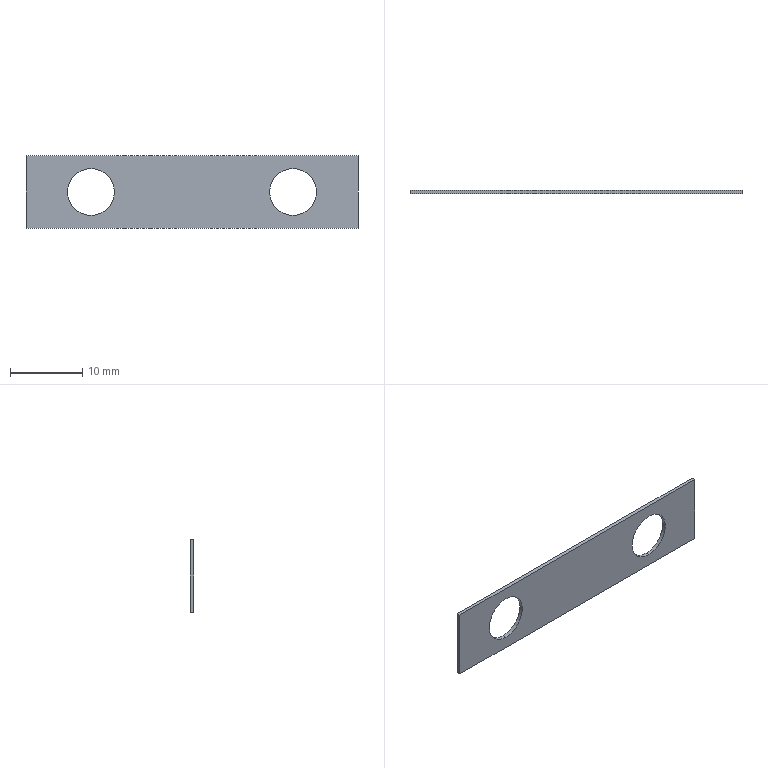Part | SolidWorks | features BaseBody 1 | 1 solid | 10 faces | box 46 x 0.5 x 10 mm | volume 196.817 mm3 | plane 6 | cylinder 4 | commonest cylinder face diameters 6.5 x4
STEP:
#1=CARTESIAN_POINT('',(14.,0.5,3.25));
#2=VERTEX_POINT('',#1);
#3=CARTESIAN_POINT('',(14.,0.5,-3.25));
#4=VERTEX_POINT('',#3);
#5=CARTESIAN_POINT('',(14.,0.5,0.));
#6=DIRECTION('',(0.,-1.,0.));
#7=DIRECTION('',(0.,0.,1.));
#8=AXIS2_PLACEMENT_3D('',#5,#6,#7);
#9=CIRCLE('',#8,3.25);
#10=EDGE_CURVE('',#2,#4,#9,.T.);
#11=ORIENTED_EDGE('',*,*,#10,.T.);
#12=CARTESIAN_POINT('',(14.,0.5,0.));
#13=DIRECTION('',(0.,-1.,0.));
#14=DIRECTION('',(0.,0.,1.));
#15=AXIS2_PLACEMENT_3D('',#12,#13,#14);
#16=CIRCLE('',#15,3.25);
#17=EDGE_CURVE('',#4,#2,#16,.T.);
#18=ORIENTED_EDGE('',*,*,#17,.T.);
#19=EDGE_LOOP('',(#11,#18));
#20=FACE_BOUND('',#19,.T.);
#21=CARTESIAN_POINT('',(-14.,0.5,3.25));
#22=VERTEX_POINT('',#21);
#23=CARTESIAN_POINT('',(-14.,0.5,-3.25));
#24=VERTEX_POINT('',#23);
#25=CARTESIAN_POINT('',(-14.,0.5,0.));
#26=DIRECTION('',(0.,-1.,0.));
#27=DIRECTION('',(0.,0.,1.));
#28=AXIS2_PLACEMENT_3D('',#25,#26,#27);
#29=CIRCLE('',#28,3.25);
#30=EDGE_CURVE('',#22,#24,#29,.T.);
#31=ORIENTED_EDGE('',*,*,#30,.T.);
#32=CARTESIAN_POINT('',(-14.,0.5,0.));
#33=DIRECTION('',(0.,-1.,0.));
#34=DIRECTION('',(0.,0.,1.));
#35=AXIS2_PLACEMENT_3D('',#32,#33,#34);
#36=CIRCLE('',#35,3.25);
#37=EDGE_CURVE('',#24,#22,#36,.T.);
#38=ORIENTED_EDGE('',*,*,#37,.T.);
#39=EDGE_LOOP('',(#31,#38));
#40=FACE_BOUND('',#39,.T.);
#41=CARTESIAN_POINT('',(23.,0.5,5.));
#42=VERTEX_POINT('',#41);
#43=CARTESIAN_POINT('',(23.,0.5,-5.));
#44=VERTEX_POINT('',#43);
#45=CARTESIAN_POINT('',(23.,0.5,-5.));
#46=DIRECTION('',(0.,0.,-1.));
#47=VECTOR('',#46,1000.);
#48=LINE('',#45,#47);
#49=EDGE_CURVE('',#42,#44,#48,.T.);
#50=ORIENTED_EDGE('',*,*,#49,.T.);
#51=CARTESIAN_POINT('',(-23.,0.5,-5.));
#52=VERTEX_POINT('',#51);
#53=CARTESIAN_POINT('',(-23.,0.5,-5.));
#54=DIRECTION('',(-1.,0.,0.));
#55=VECTOR('',#54,1000.);
#56=LINE('',#53,#55);
#57=EDGE_CURVE('',#44,#52,#56,.T.);
#58=ORIENTED_EDGE('',*,*,#57,.T.);
#59=CARTESIAN_POINT('',(-23.,0.5,5.));
#60=VERTEX_POINT('',#59);
#61=CARTESIAN_POINT('',(-23.,0.5,-5.));
#62=DIRECTION('',(0.,0.,1.));
#63=VECTOR('',#62,1000.);
#64=LINE('',#61,#63);
#65=EDGE_CURVE('',#52,#60,#64,.T.);
#66=ORIENTED_EDGE('',*,*,#65,.T.);
#67=CARTESIAN_POINT('',(-23.,0.5,5.));
#68=DIRECTION('',(1.,0.,0.));
#69=VECTOR('',#68,1000.);
#70=LINE('',#67,#69);
#71=EDGE_CURVE('',#60,#42,#70,.T.);
#72=ORIENTED_EDGE('',*,*,#71,.T.);
#73=EDGE_LOOP('',(#50,#58,#66,#72));
#74=FACE_OUTER_BOUND('',#73,.T.);
#75=CARTESIAN_POINT('',(0.,0.5,0.));
#76=DIRECTION('',(0.,1.,0.));
#77=DIRECTION('',(1.,0.,0.));
#78=AXIS2_PLACEMENT_3D('',#75,#76,#77);
#79=PLANE('',#78);
#80=ADVANCED_FACE('',(#20,#40,#74),#79,.T.);
#81=ORIENTED_EDGE('',*,*,#49,.F.);
#82=CARTESIAN_POINT('',(23.,0.,5.));
#83=VERTEX_POINT('',#82);
#84=CARTESIAN_POINT('',(23.,0.5,5.));
#85=DIRECTION('',(0.,-1.,0.));
#86=VECTOR('',#85,1000.);
#87=LINE('',#84,#86);
#88=EDGE_CURVE('',#42,#83,#87,.T.);
#89=ORIENTED_EDGE('',*,*,#88,.T.);
#90=CARTESIAN_POINT('',(23.,0.,-5.));
#91=VERTEX_POINT('',#90);
#92=CARTESIAN_POINT('',(23.,0.,0.));
#93=DIRECTION('',(0.,0.,-1.));
#94=VECTOR('',#93,1000.);
#95=LINE('',#92,#94);
#96=EDGE_CURVE('',#83,#91,#95,.T.);
#97=ORIENTED_EDGE('',*,*,#96,.T.);
#98=CARTESIAN_POINT('',(23.,0.5,-5.));
#99=DIRECTION('',(0.,1.,0.));
#100=VECTOR('',#99,1000.);
#101=LINE('',#98,#100);
#102=EDGE_CURVE('',#91,#44,#101,.T.);
#103=ORIENTED_EDGE('',*,*,#102,.T.);
#104=EDGE_LOOP('',(#81,#89,#97,#103));
#105=FACE_OUTER_BOUND('',#104,.T.);
#106=CARTESIAN_POINT('',(23.,0.5,-5.));
#107=DIRECTION('',(-1.,0.,0.));
#108=DIRECTION('',(0.,0.,1.));
#109=AXIS2_PLACEMENT_3D('',#106,#107,#108);
#110=PLANE('',#109);
#111=ADVANCED_FACE('',(#105),#110,.F.);
#112=ORIENTED_EDGE('',*,*,#57,.F.);
#113=ORIENTED_EDGE('',*,*,#102,.F.);
#114=CARTESIAN_POINT('',(-23.,0.,-5.));
#115=VERTEX_POINT('',#114);
#116=CARTESIAN_POINT('',(0.,0.,-5.));
#117=DIRECTION('',(-1.,0.,0.));
#118=VECTOR('',#117,1000.);
#119=LINE('',#116,#118);
#120=EDGE_CURVE('',#91,#115,#119,.T.);
#121=ORIENTED_EDGE('',*,*,#120,.T.);
#122=CARTESIAN_POINT('',(-23.,0.5,-5.));
#123=DIRECTION('',(0.,1.,0.));
#124=VECTOR('',#123,1000.);
#125=LINE('',#122,#124);
#126=EDGE_CURVE('',#115,#52,#125,.T.);
#127=ORIENTED_EDGE('',*,*,#126,.T.);
#128=EDGE_LOOP('',(#112,#113,#121,#127));
#129=FACE_OUTER_BOUND('',#128,.T.);
#130=CARTESIAN_POINT('',(-23.,0.5,-5.));
#131=DIRECTION('',(0.,0.,1.));
#132=DIRECTION('',(1.,0.,0.));
#133=AXIS2_PLACEMENT_3D('',#130,#131,#132);
#134=PLANE('',#133);
#135=ADVANCED_FACE('',(#129),#134,.F.);
#136=ORIENTED_EDGE('',*,*,#65,.F.);
#137=ORIENTED_EDGE('',*,*,#126,.F.);
#138=CARTESIAN_POINT('',(-23.,0.,5.));
#139=VERTEX_POINT('',#138);
#140=CARTESIAN_POINT('',(-23.,0.,0.));
#141=DIRECTION('',(0.,0.,1.));
#142=VECTOR('',#141,1000.);
#143=LINE('',#140,#142);
#144=EDGE_CURVE('',#115,#139,#143,.T.);
#145=ORIENTED_EDGE('',*,*,#144,.T.);
#146=CARTESIAN_POINT('',(-23.,0.5,5.));
#147=DIRECTION('',(0.,1.,0.));
#148=VECTOR('',#147,1000.);
#149=LINE('',#146,#148);
#150=EDGE_CURVE('',#139,#60,#149,.T.);
#151=ORIENTED_EDGE('',*,*,#150,.T.);
#152=EDGE_LOOP('',(#136,#137,#145,#151));
#153=FACE_OUTER_BOUND('',#152,.T.);
#154=CARTESIAN_POINT('',(-23.,0.5,-5.));
#155=DIRECTION('',(1.,0.,0.));
#156=DIRECTION('',(0.,1.,0.));
#157=AXIS2_PLACEMENT_3D('',#154,#155,#156);
#158=PLANE('',#157);
#159=ADVANCED_FACE('',(#153),#158,.F.);
#160=ORIENTED_EDGE('',*,*,#71,.F.);
#161=ORIENTED_EDGE('',*,*,#150,.F.);
#162=CARTESIAN_POINT('',(0.,0.,5.));
#163=DIRECTION('',(1.,0.,0.));
#164=VECTOR('',#163,1000.);
#165=LINE('',#162,#164);
#166=EDGE_CURVE('',#139,#83,#165,.T.);
#167=ORIENTED_EDGE('',*,*,#166,.T.);
#168=ORIENTED_EDGE('',*,*,#88,.F.);
#169=EDGE_LOOP('',(#160,#161,#167,#168));
#170=FACE_OUTER_BOUND('',#169,.T.);
#171=CARTESIAN_POINT('',(-23.,0.5,5.));
#172=DIRECTION('',(0.,0.,-1.));
#173=DIRECTION('',(0.,-1.,0.));
#174=AXIS2_PLACEMENT_3D('',#171,#172,#173);
#175=PLANE('',#174);
#176=ADVANCED_FACE('',(#170),#175,.F.);
#177=CARTESIAN_POINT('',(14.,0.,-3.25));
#178=VERTEX_POINT('',#177);
#179=CARTESIAN_POINT('',(14.,0.5,-3.25));
#180=DIRECTION('',(0.,1.,0.));
#181=VECTOR('',#180,1000.);
#182=LINE('',#179,#181);
#183=EDGE_CURVE('',#178,#4,#182,.T.);
#184=ORIENTED_EDGE('',*,*,#183,.F.);
#185=CARTESIAN_POINT('',(14.,0.,3.25));
#186=VERTEX_POINT('',#185);
#187=CARTESIAN_POINT('',(14.,0.,0.));
#188=DIRECTION('',(0.,-1.,0.));
#189=DIRECTION('',(0.,0.,1.));
#190=AXIS2_PLACEMENT_3D('',#187,#188,#189);
#191=CIRCLE('',#190,3.25);
#192=EDGE_CURVE('',#178,#186,#191,.T.);
#193=ORIENTED_EDGE('',*,*,#192,.T.);
#194=CARTESIAN_POINT('',(14.,0.5,3.25));
#195=DIRECTION('',(0.,1.,0.));
#196=VECTOR('',#195,1000.);
#197=LINE('',#194,#196);
#198=EDGE_CURVE('',#186,#2,#197,.T.);
#199=ORIENTED_EDGE('',*,*,#198,.T.);
#200=ORIENTED_EDGE('',*,*,#17,.F.);
#201=EDGE_LOOP('',(#184,#193,#199,#200));
#202=FACE_OUTER_BOUND('',#201,.T.);
#203=CARTESIAN_POINT('',(14.,0.5,0.));
#204=DIRECTION('',(0.,1.,0.));
#205=DIRECTION('',(0.,0.,1.));
#206=AXIS2_PLACEMENT_3D('',#203,#204,#205);
#207=CYLINDRICAL_SURFACE('',#206,3.25);
#208=ADVANCED_FACE('',(#202),#207,.F.);
#209=CARTESIAN_POINT('',(-14.,0.,-3.25));
#210=VERTEX_POINT('',#209);
#211=CARTESIAN_POINT('',(-14.,0.5,-3.25));
#212=DIRECTION('',(0.,1.,0.));
#213=VECTOR('',#212,1000.);
#214=LINE('',#211,#213);
#215=EDGE_CURVE('',#210,#24,#214,.T.);
#216=ORIENTED_EDGE('',*,*,#215,.F.);
#217=CARTESIAN_POINT('',(-14.,0.,3.25));
#218=VERTEX_POINT('',#217);
#219=CARTESIAN_POINT('',(-14.,0.,0.));
#220=DIRECTION('',(0.,-1.,0.));
#221=DIRECTION('',(0.,0.,1.));
#222=AXIS2_PLACEMENT_3D('',#219,#220,#221);
#223=CIRCLE('',#222,3.25);
#224=EDGE_CURVE('',#210,#218,#223,.T.);
#225=ORIENTED_EDGE('',*,*,#224,.T.);
#226=CARTESIAN_POINT('',(-14.,0.5,3.25));
#227=DIRECTION('',(0.,1.,0.));
#228=VECTOR('',#227,1000.);
#229=LINE('',#226,#228);
#230=EDGE_CURVE('',#218,#22,#229,.T.);
#231=ORIENTED_EDGE('',*,*,#230,.T.);
#232=ORIENTED_EDGE('',*,*,#37,.F.);
#233=EDGE_LOOP('',(#216,#225,#231,#232));
#234=FACE_OUTER_BOUND('',#233,.T.);
#235=CARTESIAN_POINT('',(-14.,0.5,0.));
#236=DIRECTION('',(0.,1.,0.));
#237=DIRECTION('',(0.,0.,1.));
#238=AXIS2_PLACEMENT_3D('',#235,#236,#237);
#239=CYLINDRICAL_SURFACE('',#238,3.25);
#240=ADVANCED_FACE('',(#234),#239,.F.);
#241=CARTESIAN_POINT('',(14.,0.,0.));
#242=DIRECTION('',(0.,-1.,0.));
#243=DIRECTION('',(0.,0.,1.));
#244=AXIS2_PLACEMENT_3D('',#241,#242,#243);
#245=CIRCLE('',#244,3.25);
#246=EDGE_CURVE('',#186,#178,#245,.T.);
#247=ORIENTED_EDGE('',*,*,#246,.F.);
#248=ORIENTED_EDGE('',*,*,#192,.F.);
#249=EDGE_LOOP('',(#247,#248));
#250=FACE_BOUND('',#249,.T.);
#251=CARTESIAN_POINT('',(-14.,0.,0.));
#252=DIRECTION('',(0.,-1.,0.));
#253=DIRECTION('',(0.,0.,1.));
#254=AXIS2_PLACEMENT_3D('',#251,#252,#253);
#255=CIRCLE('',#254,3.25);
#256=EDGE_CURVE('',#218,#210,#255,.T.);
#257=ORIENTED_EDGE('',*,*,#256,.F.);
#258=ORIENTED_EDGE('',*,*,#224,.F.);
#259=EDGE_LOOP('',(#257,#258));
#260=FACE_BOUND('',#259,.T.);
#261=ORIENTED_EDGE('',*,*,#144,.F.);
#262=ORIENTED_EDGE('',*,*,#120,.F.);
#263=ORIENTED_EDGE('',*,*,#96,.F.);
#264=ORIENTED_EDGE('',*,*,#166,.F.);
#265=EDGE_LOOP('',(#261,#262,#263,#264));
#266=FACE_OUTER_BOUND('',#265,.T.);
#267=CARTESIAN_POINT('',(0.,0.,0.));
#268=DIRECTION('',(0.,1.,0.));
#269=DIRECTION('',(1.,0.,0.));
#270=AXIS2_PLACEMENT_3D('',#267,#268,#269);
#271=PLANE('',#270);
#272=ADVANCED_FACE('',(#250,#260,#266),#271,.F.);
#273=ORIENTED_EDGE('',*,*,#246,.T.);
#274=ORIENTED_EDGE('',*,*,#183,.T.);
#275=ORIENTED_EDGE('',*,*,#10,.F.);
#276=ORIENTED_EDGE('',*,*,#198,.F.);
#277=EDGE_LOOP('',(#273,#274,#275,#276));
#278=FACE_OUTER_BOUND('',#277,.T.);
#279=CARTESIAN_POINT('',(14.,0.5,0.));
#280=DIRECTION('',(0.,1.,0.));
#281=DIRECTION('',(0.,0.,1.));
#282=AXIS2_PLACEMENT_3D('',#279,#280,#281);
#283=CYLINDRICAL_SURFACE('',#282,3.25);
#284=ADVANCED_FACE('',(#278),#283,.F.);
#285=ORIENTED_EDGE('',*,*,#256,.T.);
#286=ORIENTED_EDGE('',*,*,#215,.T.);
#287=ORIENTED_EDGE('',*,*,#30,.F.);
#288=ORIENTED_EDGE('',*,*,#230,.F.);
#289=EDGE_LOOP('',(#285,#286,#287,#288));
#290=FACE_OUTER_BOUND('',#289,.T.);
#291=CARTESIAN_POINT('',(-14.,0.5,0.));
#292=DIRECTION('',(0.,1.,0.));
#293=DIRECTION('',(0.,0.,1.));
#294=AXIS2_PLACEMENT_3D('',#291,#292,#293);
#295=CYLINDRICAL_SURFACE('',#294,3.25);
#296=ADVANCED_FACE('',(#290),#295,.F.);
#297=CLOSED_SHELL('',(#80,#111,#135,#159,#176,#208,#240,#272,#284,#296));
#298=MANIFOLD_SOLID_BREP('',#297);
#299=CARTESIAN_POINT('',(0.,0.,0.));
#300=DIRECTION('',(0.,0.,1.));
#301=DIRECTION('',(1.,0.,0.));
#302=AXIS2_PLACEMENT_3D('',#299,#300,#301);
#303=(LENGTH_UNIT()NAMED_UNIT(*)SI_UNIT(.MILLI.,.METRE.));
#304=UNCERTAINTY_MEASURE_WITH_UNIT(LENGTH_MEASURE(0.00001),#303,'','');
#305=(NAMED_UNIT(*)PLANE_ANGLE_UNIT()SI_UNIT($,.RADIAN.));
#306=(NAMED_UNIT(*)SI_UNIT($,.STERADIAN.)SOLID_ANGLE_UNIT());
#307=(GEOMETRIC_REPRESENTATION_CONTEXT(3)GLOBAL_UNCERTAINTY_ASSIGNED_CONTEXT((#304))GLOBAL_UNIT_ASSIGNED_CONTEXT((#303,#305,#306))REPRESENTATION_CONTEXT('',''));
#308=ADVANCED_BREP_SHAPE_REPRESENTATION('',(#298,#302),#307);